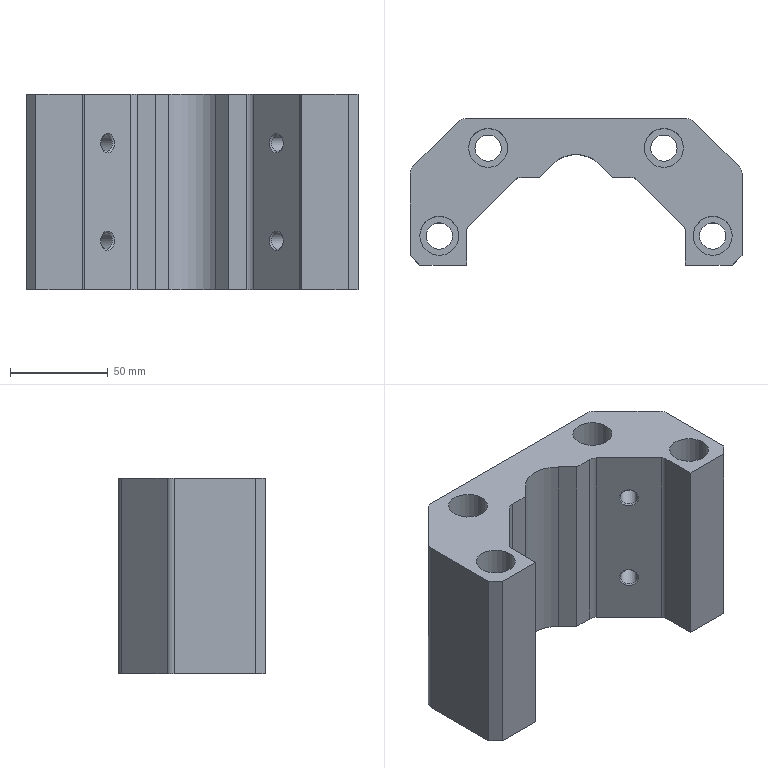Part | NX | features LB-9 2 | 1 solid | 52 faces | box 170 x 75 x 100 mm | volume 629709 mm3 | plane 23 | cylinder 21 | cone 8 | commonest cylinder face diameters 10 x6 8.506 x4 13.5 x4 20 x4 6 x2 34 x1
STEP:
#1=CARTESIAN_POINT('',(3387.594,-1089.122,888.716));
#2=VERTEX_POINT('',#1);
#3=CARTESIAN_POINT('',(3377.594,-1089.122,888.716));
#4=DIRECTION('',(0.,0.,1.));
#5=DIRECTION('',(1.,0.,0.));
#6=AXIS2_PLACEMENT_3D('',#3,#4,#5);
#7=CIRCLE('',#6,10.);
#8=EDGE_CURVE('',#2,#2,#7,.T.);
#9=ORIENTED_EDGE('',*,*,#8,.F.);
#10=EDGE_LOOP('',(#9));
#11=FACE_BOUND('',#10,.T.);
#12=CARTESIAN_POINT('',(3272.594,-1044.122,888.716));
#13=VERTEX_POINT('',#12);
#14=CARTESIAN_POINT('',(3262.594,-1044.122,888.716));
#15=DIRECTION('',(0.,0.,1.));
#16=DIRECTION('',(1.,0.,0.));
#17=AXIS2_PLACEMENT_3D('',#14,#15,#16);
#18=CIRCLE('',#17,10.);
#19=EDGE_CURVE('',#13,#13,#18,.T.);
#20=ORIENTED_EDGE('',*,*,#19,.F.);
#21=EDGE_LOOP('',(#20));
#22=FACE_BOUND('',#21,.T.);
#23=CARTESIAN_POINT('',(3362.594,-1044.122,888.716));
#24=VERTEX_POINT('',#23);
#25=CARTESIAN_POINT('',(3352.594,-1044.122,888.716));
#26=DIRECTION('',(0.,0.,1.));
#27=DIRECTION('',(1.,0.,0.));
#28=AXIS2_PLACEMENT_3D('',#25,#26,#27);
#29=CIRCLE('',#28,10.);
#30=EDGE_CURVE('',#24,#24,#29,.T.);
#31=ORIENTED_EDGE('',*,*,#30,.F.);
#32=EDGE_LOOP('',(#31));
#33=FACE_BOUND('',#32,.T.);
#34=CARTESIAN_POINT('',(3247.594,-1089.122,888.716));
#35=VERTEX_POINT('',#34);
#36=CARTESIAN_POINT('',(3237.594,-1089.122,888.716));
#37=DIRECTION('',(0.,0.,1.));
#38=DIRECTION('',(1.,0.,0.));
#39=AXIS2_PLACEMENT_3D('',#36,#37,#38);
#40=CIRCLE('',#39,10.);
#41=EDGE_CURVE('',#35,#35,#40,.T.);
#42=ORIENTED_EDGE('',*,*,#41,.F.);
#43=EDGE_LOOP('',(#42));
#44=FACE_BOUND('',#43,.T.);
#45=CARTESIAN_POINT('',(3392.594,-1099.122,888.716));
#46=VERTEX_POINT('',#45);
#47=CARTESIAN_POINT('',(3392.594,-1057.406,888.716));
#48=VERTEX_POINT('',#47);
#49=CARTESIAN_POINT('',(3392.594,-1019.122,888.716));
#50=DIRECTION('',(0.,1.,0.));
#51=VECTOR('',#50,1000.);
#52=LINE('',#49,#51);
#53=EDGE_CURVE('',#46,#48,#52,.T.);
#54=ORIENTED_EDGE('',*,*,#53,.T.);
#55=CARTESIAN_POINT('',(3391.129,-1053.871,888.716));
#56=VERTEX_POINT('',#55);
#57=CARTESIAN_POINT('',(3387.594,-1057.406,888.716));
#58=DIRECTION('',(0.,0.,1.));
#59=DIRECTION('',(1.,0.,0.));
#60=AXIS2_PLACEMENT_3D('',#57,#58,#59);
#61=CIRCLE('',#60,5.);
#62=EDGE_CURVE('',#48,#56,#61,.T.);
#63=ORIENTED_EDGE('',*,*,#62,.T.);
#64=CARTESIAN_POINT('',(3367.845,-1030.587,888.716));
#65=VERTEX_POINT('',#64);
#66=CARTESIAN_POINT('',(3138.314,-801.055,888.716));
#67=DIRECTION('',(-0.7071,0.7071,0.));
#68=VECTOR('',#67,1000.);
#69=LINE('',#66,#68);
#70=EDGE_CURVE('',#56,#65,#69,.T.);
#71=ORIENTED_EDGE('',*,*,#70,.T.);
#72=CARTESIAN_POINT('',(3364.31,-1029.122,888.716));
#73=VERTEX_POINT('',#72);
#74=CARTESIAN_POINT('',(3364.31,-1034.122,888.716));
#75=DIRECTION('',(0.,0.,1.));
#76=DIRECTION('',(1.,0.,0.));
#77=AXIS2_PLACEMENT_3D('',#74,#75,#76);
#78=CIRCLE('',#77,5.);
#79=EDGE_CURVE('',#65,#73,#78,.T.);
#80=ORIENTED_EDGE('',*,*,#79,.T.);
#81=CARTESIAN_POINT('',(3250.878,-1029.122,888.716));
#82=VERTEX_POINT('',#81);
#83=CARTESIAN_POINT('',(3237.747,-1029.122,888.716));
#84=DIRECTION('',(1.,0.,0.));
#85=VECTOR('',#84,1000.);
#86=LINE('',#83,#85);
#87=EDGE_CURVE('',#82,#73,#86,.T.);
#88=ORIENTED_EDGE('',*,*,#87,.F.);
#89=CARTESIAN_POINT('',(3247.343,-1030.587,888.716));
#90=VERTEX_POINT('',#89);
#91=CARTESIAN_POINT('',(3250.878,-1034.122,888.716));
#92=DIRECTION('',(0.,0.,1.));
#93=DIRECTION('',(1.,0.,0.));
#94=AXIS2_PLACEMENT_3D('',#91,#92,#93);
#95=CIRCLE('',#94,5.);
#96=EDGE_CURVE('',#82,#90,#95,.T.);
#97=ORIENTED_EDGE('',*,*,#96,.T.);
#98=CARTESIAN_POINT('',(3224.058,-1053.871,888.716));
#99=VERTEX_POINT('',#98);
#100=CARTESIAN_POINT('',(3407.027,-870.902,888.716));
#101=DIRECTION('',(-0.7071,-0.7071,0.));
#102=VECTOR('',#101,1000.);
#103=LINE('',#100,#102);
#104=EDGE_CURVE('',#90,#99,#103,.T.);
#105=ORIENTED_EDGE('',*,*,#104,.T.);
#106=CARTESIAN_POINT('',(3222.594,-1057.406,888.716));
#107=VERTEX_POINT('',#106);
#108=CARTESIAN_POINT('',(3227.594,-1057.406,888.716));
#109=DIRECTION('',(0.,0.,1.));
#110=DIRECTION('',(1.,0.,0.));
#111=AXIS2_PLACEMENT_3D('',#108,#109,#110);
#112=CIRCLE('',#111,5.);
#113=EDGE_CURVE('',#99,#107,#112,.T.);
#114=ORIENTED_EDGE('',*,*,#113,.T.);
#115=CARTESIAN_POINT('',(3222.594,-1099.122,888.716));
#116=VERTEX_POINT('',#115);
#117=CARTESIAN_POINT('',(3222.594,-701.622,888.716));
#118=DIRECTION('',(0.,-1.,0.));
#119=VECTOR('',#118,1000.);
#120=LINE('',#117,#119);
#121=EDGE_CURVE('',#107,#116,#120,.T.);
#122=ORIENTED_EDGE('',*,*,#121,.T.);
#123=CARTESIAN_POINT('',(3227.594,-1104.122,888.716));
#124=VERTEX_POINT('',#123);
#125=CARTESIAN_POINT('',(3023.92,-900.449,888.716));
#126=DIRECTION('',(0.7071,-0.7071,0.));
#127=VECTOR('',#126,1000.);
#128=LINE('',#125,#127);
#129=EDGE_CURVE('',#116,#124,#128,.T.);
#130=ORIENTED_EDGE('',*,*,#129,.T.);
#131=CARTESIAN_POINT('',(3251.594,-1104.122,888.716));
#132=VERTEX_POINT('',#131);
#133=CARTESIAN_POINT('',(4385.094,-1104.122,888.716));
#134=DIRECTION('',(-1.,0.,0.));
#135=VECTOR('',#134,1000.);
#136=LINE('',#133,#135);
#137=EDGE_CURVE('',#132,#124,#136,.T.);
#138=ORIENTED_EDGE('',*,*,#137,.F.);
#139=CARTESIAN_POINT('',(3251.594,-1086.365,888.716));
#140=VERTEX_POINT('',#139);
#141=CARTESIAN_POINT('',(3251.594,-701.622,888.716));
#142=DIRECTION('',(0.,-1.,0.));
#143=VECTOR('',#142,1000.);
#144=LINE('',#141,#143);
#145=EDGE_CURVE('',#140,#132,#144,.T.);
#146=ORIENTED_EDGE('',*,*,#145,.F.);
#147=CARTESIAN_POINT('',(3252.473,-1084.243,888.716));
#148=VERTEX_POINT('',#147);
#149=CARTESIAN_POINT('',(3254.594,-1086.365,888.716));
#150=DIRECTION('',(0.,0.,-1.));
#151=DIRECTION('',(1.,0.,0.));
#152=AXIS2_PLACEMENT_3D('',#149,#150,#151);
#153=CIRCLE('',#152,3.);
#154=EDGE_CURVE('',#140,#148,#153,.T.);
#155=ORIENTED_EDGE('',*,*,#154,.T.);
#156=CARTESIAN_POINT('',(3276.129,-1060.587,888.716));
#157=VERTEX_POINT('',#156);
#158=CARTESIAN_POINT('',(3428.92,-907.796,888.716));
#159=DIRECTION('',(-0.7071,-0.7071,0.));
#160=VECTOR('',#159,1000.);
#161=LINE('',#158,#160);
#162=EDGE_CURVE('',#157,#148,#161,.T.);
#163=ORIENTED_EDGE('',*,*,#162,.F.);
#164=CARTESIAN_POINT('',(3279.665,-1059.122,888.716));
#165=VERTEX_POINT('',#164);
#166=CARTESIAN_POINT('',(3279.665,-1064.122,888.716));
#167=DIRECTION('',(0.,0.,-1.));
#168=DIRECTION('',(1.,0.,0.));
#169=AXIS2_PLACEMENT_3D('',#166,#167,#168);
#170=CIRCLE('',#169,5.);
#171=EDGE_CURVE('',#157,#165,#170,.T.);
#172=ORIENTED_EDGE('',*,*,#171,.T.);
#173=CARTESIAN_POINT('',(3288.908,-1059.122,888.716));
#174=VERTEX_POINT('',#173);
#175=CARTESIAN_POINT('',(3237.747,-1059.122,888.716));
#176=DIRECTION('',(-1.,0.,0.));
#177=VECTOR('',#176,1000.);
#178=LINE('',#175,#177);
#179=EDGE_CURVE('',#174,#165,#178,.T.);
#180=ORIENTED_EDGE('',*,*,#179,.F.);
#181=CARTESIAN_POINT('',(3295.573,-1052.457,888.716));
#182=VERTEX_POINT('',#181);
#183=CARTESIAN_POINT('',(3442.077,-905.952,888.716));
#184=DIRECTION('',(0.7071,0.7071,0.));
#185=VECTOR('',#184,1000.);
#186=LINE('',#183,#185);
#187=EDGE_CURVE('',#174,#182,#186,.T.);
#188=ORIENTED_EDGE('',*,*,#187,.T.);
#189=CARTESIAN_POINT('',(3319.615,-1052.457,888.716));
#190=VERTEX_POINT('',#189);
#191=CARTESIAN_POINT('',(3307.594,-1064.477,888.716));
#192=DIRECTION('',(0.,0.,1.));
#193=DIRECTION('',(1.,0.,0.));
#194=AXIS2_PLACEMENT_3D('',#191,#192,#193);
#195=CIRCLE('',#194,17.);
#196=EDGE_CURVE('',#190,#182,#195,.T.);
#197=ORIENTED_EDGE('',*,*,#196,.F.);
#198=CARTESIAN_POINT('',(3326.28,-1059.122,888.716));
#199=VERTEX_POINT('',#198);
#200=CARTESIAN_POINT('',(3103.264,-836.105,888.716));
#201=DIRECTION('',(0.7071,-0.7071,0.));
#202=VECTOR('',#201,1000.);
#203=LINE('',#200,#202);
#204=EDGE_CURVE('',#190,#199,#203,.T.);
#205=ORIENTED_EDGE('',*,*,#204,.T.);
#206=CARTESIAN_POINT('',(3335.523,-1059.122,888.716));
#207=VERTEX_POINT('',#206);
#208=CARTESIAN_POINT('',(3237.747,-1059.122,888.716));
#209=DIRECTION('',(-1.,0.,0.));
#210=VECTOR('',#209,1000.);
#211=LINE('',#208,#210);
#212=EDGE_CURVE('',#207,#199,#211,.T.);
#213=ORIENTED_EDGE('',*,*,#212,.F.);
#214=CARTESIAN_POINT('',(3339.058,-1060.587,888.716));
#215=VERTEX_POINT('',#214);
#216=CARTESIAN_POINT('',(3335.523,-1064.122,888.716));
#217=DIRECTION('',(0.,0.,-1.));
#218=DIRECTION('',(1.,0.,0.));
#219=AXIS2_PLACEMENT_3D('',#216,#217,#218);
#220=CIRCLE('',#219,5.);
#221=EDGE_CURVE('',#207,#215,#220,.T.);
#222=ORIENTED_EDGE('',*,*,#221,.T.);
#223=CARTESIAN_POINT('',(3362.715,-1084.243,888.716));
#224=VERTEX_POINT('',#223);
#225=CARTESIAN_POINT('',(3347.594,-1069.122,888.716));
#226=DIRECTION('',(-0.7071,0.7071,0.));
#227=VECTOR('',#226,1000.);
#228=LINE('',#225,#227);
#229=EDGE_CURVE('',#224,#215,#228,.T.);
#230=ORIENTED_EDGE('',*,*,#229,.F.);
#231=CARTESIAN_POINT('',(3363.594,-1086.365,888.716));
#232=VERTEX_POINT('',#231);
#233=CARTESIAN_POINT('',(3360.594,-1086.365,888.716));
#234=DIRECTION('',(0.,0.,-1.));
#235=DIRECTION('',(1.,0.,0.));
#236=AXIS2_PLACEMENT_3D('',#233,#234,#235);
#237=CIRCLE('',#236,3.);
#238=EDGE_CURVE('',#224,#232,#237,.T.);
#239=ORIENTED_EDGE('',*,*,#238,.T.);
#240=CARTESIAN_POINT('',(3363.594,-1104.122,888.716));
#241=VERTEX_POINT('',#240);
#242=CARTESIAN_POINT('',(3363.594,-1061.622,888.716));
#243=DIRECTION('',(0.,-1.,0.));
#244=VECTOR('',#243,1000.);
#245=LINE('',#242,#244);
#246=EDGE_CURVE('',#232,#241,#245,.T.);
#247=ORIENTED_EDGE('',*,*,#246,.T.);
#248=CARTESIAN_POINT('',(3387.594,-1104.122,888.716));
#249=VERTEX_POINT('',#248);
#250=CARTESIAN_POINT('',(4387.594,-1104.122,888.716));
#251=DIRECTION('',(-1.,0.,0.));
#252=VECTOR('',#251,1000.);
#253=LINE('',#250,#252);
#254=EDGE_CURVE('',#249,#241,#253,.T.);
#255=ORIENTED_EDGE('',*,*,#254,.F.);
#256=CARTESIAN_POINT('',(3521.42,-970.296,888.716));
#257=DIRECTION('',(0.7071,0.7071,0.));
#258=VECTOR('',#257,1000.);
#259=LINE('',#256,#258);
#260=EDGE_CURVE('',#249,#46,#259,.T.);
#261=ORIENTED_EDGE('',*,*,#260,.T.);
#262=EDGE_LOOP('',(#54,#63,#71,#80,#88,#97,#105,#114,#122,#130,#138,#146,#155,#163,#172,#180,#188,#197,#205,#213,#222,#230,#239,#247,#255,#261));
#263=FACE_BOUND('',#262,.T.);
#264=CARTESIAN_POINT('',(3237.747,-701.622,888.716));
#265=DIRECTION('',(0.,0.,1.));
#266=DIRECTION('',(-1.,0.,0.));
#267=AXIS2_PLACEMENT_3D('',#264,#265,#266);
#268=PLANE('',#267);
#269=ADVANCED_FACE('',(#11,#22,#33,#44,#263),#268,.T.);
#270=CARTESIAN_POINT('',(3384.344,-1089.122,788.716));
#271=VERTEX_POINT('',#270);
#272=CARTESIAN_POINT('',(3377.594,-1089.122,788.716));
#273=DIRECTION('',(0.,0.,1.));
#274=DIRECTION('',(1.,0.,0.));
#275=AXIS2_PLACEMENT_3D('',#272,#273,#274);
#276=CIRCLE('',#275,6.75);
#277=EDGE_CURVE('',#271,#271,#276,.T.);
#278=ORIENTED_EDGE('',*,*,#277,.T.);
#279=EDGE_LOOP('',(#278));
#280=FACE_BOUND('',#279,.T.);
#281=CARTESIAN_POINT('',(3269.344,-1044.122,788.716));
#282=VERTEX_POINT('',#281);
#283=CARTESIAN_POINT('',(3262.594,-1044.122,788.716));
#284=DIRECTION('',(0.,0.,1.));
#285=DIRECTION('',(1.,0.,0.));
#286=AXIS2_PLACEMENT_3D('',#283,#284,#285);
#287=CIRCLE('',#286,6.75);
#288=EDGE_CURVE('',#282,#282,#287,.T.);
#289=ORIENTED_EDGE('',*,*,#288,.T.);
#290=EDGE_LOOP('',(#289));
#291=FACE_BOUND('',#290,.T.);
#292=CARTESIAN_POINT('',(3359.344,-1044.122,788.716));
#293=VERTEX_POINT('',#292);
#294=CARTESIAN_POINT('',(3352.594,-1044.122,788.716));
#295=DIRECTION('',(0.,0.,1.));
#296=DIRECTION('',(1.,0.,0.));
#297=AXIS2_PLACEMENT_3D('',#294,#295,#296);
#298=CIRCLE('',#297,6.75);
#299=EDGE_CURVE('',#293,#293,#298,.T.);
#300=ORIENTED_EDGE('',*,*,#299,.T.);
#301=EDGE_LOOP('',(#300));
#302=FACE_BOUND('',#301,.T.);
#303=CARTESIAN_POINT('',(3244.344,-1089.122,788.716));
#304=VERTEX_POINT('',#303);
#305=CARTESIAN_POINT('',(3237.594,-1089.122,788.716));
#306=DIRECTION('',(0.,0.,1.));
#307=DIRECTION('',(1.,0.,0.));
#308=AXIS2_PLACEMENT_3D('',#305,#306,#307);
#309=CIRCLE('',#308,6.75);
#310=EDGE_CURVE('',#304,#304,#309,.T.);
#311=ORIENTED_EDGE('',*,*,#310,.T.);
#312=EDGE_LOOP('',(#311));
#313=FACE_BOUND('',#312,.T.);
#314=CARTESIAN_POINT('',(3367.845,-1030.587,788.716));
#315=VERTEX_POINT('',#314);
#316=CARTESIAN_POINT('',(3391.129,-1053.871,788.716));
#317=VERTEX_POINT('',#316);
#318=CARTESIAN_POINT('',(3376.987,-1039.729,788.716));
#319=DIRECTION('',(0.7071,-0.7071,0.));
#320=VECTOR('',#319,1000.);
#321=LINE('',#318,#320);
#322=EDGE_CURVE('',#315,#317,#321,.T.);
#323=ORIENTED_EDGE('',*,*,#322,.T.);
#324=CARTESIAN_POINT('',(3392.594,-1057.406,788.716));
#325=VERTEX_POINT('',#324);
#326=CARTESIAN_POINT('',(3387.594,-1057.406,788.716));
#327=DIRECTION('',(0.,0.,-1.));
#328=DIRECTION('',(1.,0.,0.));
#329=AXIS2_PLACEMENT_3D('',#326,#327,#328);
#330=CIRCLE('',#329,5.);
#331=EDGE_CURVE('',#317,#325,#330,.T.);
#332=ORIENTED_EDGE('',*,*,#331,.T.);
#333=CARTESIAN_POINT('',(3392.594,-1099.122,788.716));
#334=VERTEX_POINT('',#333);
#335=CARTESIAN_POINT('',(3392.594,-299.122,788.716));
#336=DIRECTION('',(0.,-1.,0.));
#337=VECTOR('',#336,1000.);
#338=LINE('',#335,#337);
#339=EDGE_CURVE('',#325,#334,#338,.T.);
#340=ORIENTED_EDGE('',*,*,#339,.T.);
#341=CARTESIAN_POINT('',(3387.594,-1104.122,788.716));
#342=VERTEX_POINT('',#341);
#343=CARTESIAN_POINT('',(3392.594,-1099.122,788.716));
#344=DIRECTION('',(-0.7071,-0.7071,0.));
#345=VECTOR('',#344,1000.);
#346=LINE('',#343,#345);
#347=EDGE_CURVE('',#334,#342,#346,.T.);
#348=ORIENTED_EDGE('',*,*,#347,.T.);
#349=CARTESIAN_POINT('',(3363.594,-1104.122,788.716));
#350=VERTEX_POINT('',#349);
#351=CARTESIAN_POINT('',(3660.094,-1104.122,788.716));
#352=DIRECTION('',(1.,0.,0.));
#353=VECTOR('',#352,1000.);
#354=LINE('',#351,#353);
#355=EDGE_CURVE('',#350,#342,#354,.T.);
#356=ORIENTED_EDGE('',*,*,#355,.F.);
#357=CARTESIAN_POINT('',(3363.594,-1086.365,788.716));
#358=VERTEX_POINT('',#357);
#359=CARTESIAN_POINT('',(3363.594,-299.122,788.716));
#360=DIRECTION('',(0.,1.,0.));
#361=VECTOR('',#360,1000.);
#362=LINE('',#359,#361);
#363=EDGE_CURVE('',#350,#358,#362,.T.);
#364=ORIENTED_EDGE('',*,*,#363,.T.);
#365=CARTESIAN_POINT('',(3362.715,-1084.243,788.716));
#366=VERTEX_POINT('',#365);
#367=CARTESIAN_POINT('',(3360.594,-1086.365,788.716));
#368=DIRECTION('',(0.,0.,1.));
#369=DIRECTION('',(1.,0.,0.));
#370=AXIS2_PLACEMENT_3D('',#367,#368,#369);
#371=CIRCLE('',#370,3.);
#372=EDGE_CURVE('',#358,#366,#371,.T.);
#373=ORIENTED_EDGE('',*,*,#372,.T.);
#374=CARTESIAN_POINT('',(3339.058,-1060.587,788.716));
#375=VERTEX_POINT('',#374);
#376=CARTESIAN_POINT('',(3347.594,-1069.122,788.716));
#377=DIRECTION('',(-0.7071,0.7071,0.));
#378=VECTOR('',#377,1000.);
#379=LINE('',#376,#378);
#380=EDGE_CURVE('',#366,#375,#379,.T.);
#381=ORIENTED_EDGE('',*,*,#380,.T.);
#382=CARTESIAN_POINT('',(3335.523,-1059.122,788.716));
#383=VERTEX_POINT('',#382);
#384=CARTESIAN_POINT('',(3335.523,-1064.122,788.716));
#385=DIRECTION('',(0.,0.,1.));
#386=DIRECTION('',(1.,0.,0.));
#387=AXIS2_PLACEMENT_3D('',#384,#385,#386);
#388=CIRCLE('',#387,5.);
#389=EDGE_CURVE('',#375,#383,#388,.T.);
#390=ORIENTED_EDGE('',*,*,#389,.T.);
#391=CARTESIAN_POINT('',(3326.28,-1059.122,788.716));
#392=VERTEX_POINT('',#391);
#393=CARTESIAN_POINT('',(4922.709,-1059.122,788.716));
#394=DIRECTION('',(1.,0.,0.));
#395=VECTOR('',#394,1000.);
#396=LINE('',#393,#395);
#397=EDGE_CURVE('',#392,#383,#396,.T.);
#398=ORIENTED_EDGE('',*,*,#397,.F.);
#399=CARTESIAN_POINT('',(3319.615,-1052.457,788.716));
#400=VERTEX_POINT('',#399);
#401=CARTESIAN_POINT('',(3105.687,-838.529,788.716));
#402=DIRECTION('',(0.7071,-0.7071,0.));
#403=VECTOR('',#402,1000.);
#404=LINE('',#401,#403);
#405=EDGE_CURVE('',#400,#392,#404,.T.);
#406=ORIENTED_EDGE('',*,*,#405,.F.);
#407=CARTESIAN_POINT('',(3295.573,-1052.457,788.716));
#408=VERTEX_POINT('',#407);
#409=CARTESIAN_POINT('',(3307.594,-1064.477,788.716));
#410=DIRECTION('',(0.,0.,1.));
#411=DIRECTION('',(1.,0.,0.));
#412=AXIS2_PLACEMENT_3D('',#409,#410,#411);
#413=CIRCLE('',#412,17.);
#414=EDGE_CURVE('',#400,#408,#413,.T.);
#415=ORIENTED_EDGE('',*,*,#414,.T.);
#416=CARTESIAN_POINT('',(3288.908,-1059.122,788.716));
#417=VERTEX_POINT('',#416);
#418=CARTESIAN_POINT('',(3847.001,-501.029,788.716));
#419=DIRECTION('',(0.7071,0.7071,0.));
#420=VECTOR('',#419,1000.);
#421=LINE('',#418,#420);
#422=EDGE_CURVE('',#417,#408,#421,.T.);
#423=ORIENTED_EDGE('',*,*,#422,.F.);
#424=CARTESIAN_POINT('',(3279.665,-1059.122,788.716));
#425=VERTEX_POINT('',#424);
#426=CARTESIAN_POINT('',(4922.709,-1059.122,788.716));
#427=DIRECTION('',(1.,0.,0.));
#428=VECTOR('',#427,1000.);
#429=LINE('',#426,#428);
#430=EDGE_CURVE('',#425,#417,#429,.T.);
#431=ORIENTED_EDGE('',*,*,#430,.F.);
#432=CARTESIAN_POINT('',(3276.129,-1060.587,788.716));
#433=VERTEX_POINT('',#432);
#434=CARTESIAN_POINT('',(3279.665,-1064.122,788.716));
#435=DIRECTION('',(0.,0.,1.));
#436=DIRECTION('',(1.,0.,0.));
#437=AXIS2_PLACEMENT_3D('',#434,#435,#436);
#438=CIRCLE('',#437,5.);
#439=EDGE_CURVE('',#425,#433,#438,.T.);
#440=ORIENTED_EDGE('',*,*,#439,.T.);
#441=CARTESIAN_POINT('',(3252.473,-1084.243,788.716));
#442=VERTEX_POINT('',#441);
#443=CARTESIAN_POINT('',(3833.844,-502.872,788.716));
#444=DIRECTION('',(-0.7071,-0.7071,0.));
#445=VECTOR('',#444,1000.);
#446=LINE('',#443,#445);
#447=EDGE_CURVE('',#433,#442,#446,.T.);
#448=ORIENTED_EDGE('',*,*,#447,.T.);
#449=CARTESIAN_POINT('',(3251.594,-1086.365,788.716));
#450=VERTEX_POINT('',#449);
#451=CARTESIAN_POINT('',(3254.594,-1086.365,788.716));
#452=DIRECTION('',(0.,0.,1.));
#453=DIRECTION('',(1.,0.,0.));
#454=AXIS2_PLACEMENT_3D('',#451,#452,#453);
#455=CIRCLE('',#454,3.);
#456=EDGE_CURVE('',#442,#450,#455,.T.);
#457=ORIENTED_EDGE('',*,*,#456,.T.);
#458=CARTESIAN_POINT('',(3251.594,-1104.122,788.716));
#459=VERTEX_POINT('',#458);
#460=CARTESIAN_POINT('',(3251.594,-1061.622,788.716));
#461=DIRECTION('',(0.,1.,0.));
#462=VECTOR('',#461,1000.);
#463=LINE('',#460,#462);
#464=EDGE_CURVE('',#459,#450,#463,.T.);
#465=ORIENTED_EDGE('',*,*,#464,.F.);
#466=CARTESIAN_POINT('',(3227.594,-1104.122,788.716));
#467=VERTEX_POINT('',#466);
#468=CARTESIAN_POINT('',(4385.094,-1104.122,788.716));
#469=DIRECTION('',(-1.,0.,0.));
#470=VECTOR('',#469,1000.);
#471=LINE('',#468,#470);
#472=EDGE_CURVE('',#459,#467,#471,.T.);
#473=ORIENTED_EDGE('',*,*,#472,.T.);
#474=CARTESIAN_POINT('',(3222.594,-1099.122,788.716));
#475=VERTEX_POINT('',#474);
#476=CARTESIAN_POINT('',(3227.594,-1104.122,788.716));
#477=DIRECTION('',(-0.7071,0.7071,0.));
#478=VECTOR('',#477,1000.);
#479=LINE('',#476,#478);
#480=EDGE_CURVE('',#467,#475,#479,.T.);
#481=ORIENTED_EDGE('',*,*,#480,.T.);
#482=CARTESIAN_POINT('',(3222.594,-1057.406,788.716));
#483=VERTEX_POINT('',#482);
#484=CARTESIAN_POINT('',(3222.594,-299.122,788.716));
#485=DIRECTION('',(0.,-1.,0.));
#486=VECTOR('',#485,1000.);
#487=LINE('',#484,#486);
#488=EDGE_CURVE('',#483,#475,#487,.T.);
#489=ORIENTED_EDGE('',*,*,#488,.F.);
#490=CARTESIAN_POINT('',(3224.058,-1053.871,788.716));
#491=VERTEX_POINT('',#490);
#492=CARTESIAN_POINT('',(3227.594,-1057.406,788.716));
#493=DIRECTION('',(0.,0.,-1.));
#494=DIRECTION('',(1.,0.,0.));
#495=AXIS2_PLACEMENT_3D('',#492,#493,#494);
#496=CIRCLE('',#495,5.);
#497=EDGE_CURVE('',#483,#491,#496,.T.);
#498=ORIENTED_EDGE('',*,*,#497,.T.);
#499=CARTESIAN_POINT('',(3247.343,-1030.587,788.716));
#500=VERTEX_POINT('',#499);
#501=CARTESIAN_POINT('',(3233.201,-1044.729,788.716));
#502=DIRECTION('',(0.7071,0.7071,0.));
#503=VECTOR('',#502,1000.);
#504=LINE('',#501,#503);
#505=EDGE_CURVE('',#491,#500,#504,.T.);
#506=ORIENTED_EDGE('',*,*,#505,.T.);
#507=CARTESIAN_POINT('',(3250.878,-1029.122,788.716));
#508=VERTEX_POINT('',#507);
#509=CARTESIAN_POINT('',(3250.878,-1034.122,788.716));
#510=DIRECTION('',(0.,0.,-1.));
#511=DIRECTION('',(1.,0.,0.));
#512=AXIS2_PLACEMENT_3D('',#509,#510,#511);
#513=CIRCLE('',#512,5.);
#514=EDGE_CURVE('',#500,#508,#513,.T.);
#515=ORIENTED_EDGE('',*,*,#514,.T.);
#516=CARTESIAN_POINT('',(3364.31,-1029.122,788.716));
#517=VERTEX_POINT('',#516);
#518=CARTESIAN_POINT('',(3645.094,-1029.122,788.716));
#519=DIRECTION('',(1.,0.,0.));
#520=VECTOR('',#519,1000.);
#521=LINE('',#518,#520);
#522=EDGE_CURVE('',#508,#517,#521,.T.);
#523=ORIENTED_EDGE('',*,*,#522,.T.);
#524=CARTESIAN_POINT('',(3364.31,-1034.122,788.716));
#525=DIRECTION('',(0.,0.,-1.));
#526=DIRECTION('',(1.,0.,0.));
#527=AXIS2_PLACEMENT_3D('',#524,#525,#526);
#528=CIRCLE('',#527,5.);
#529=EDGE_CURVE('',#517,#315,#528,.T.);
#530=ORIENTED_EDGE('',*,*,#529,.T.);
#531=EDGE_LOOP('',(#323,#332,#340,#348,#356,#364,#373,#381,#390,#398,#406,#415,#423,#431,#440,#448,#457,#465,#473,#481,#489,#498,#506,#515,#523,#530));
#532=FACE_BOUND('',#531,.T.);
#533=CARTESIAN_POINT('',(3645.094,-299.122,788.716));
#534=DIRECTION('',(0.,0.,1.));
#535=DIRECTION('',(-1.,0.,0.));
#536=AXIS2_PLACEMENT_3D('',#533,#534,#535);
#537=PLANE('',#536);
#538=ADVANCED_FACE('',(#280,#291,#302,#313,#532),#537,.F.);
#539=CARTESIAN_POINT('',(3326.28,-1059.122,473.116));
#540=DIRECTION('',(0.,0.,1.));
#541=VECTOR('',#540,1000.);
#542=LINE('',#539,#541);
#543=EDGE_CURVE('',#392,#199,#542,.T.);
#544=ORIENTED_EDGE('',*,*,#543,.F.);
#545=ORIENTED_EDGE('',*,*,#397,.T.);
#546=CARTESIAN_POINT('',(3335.523,-1059.122,473.116));
#547=DIRECTION('',(0.,0.,1.));
#548=VECTOR('',#547,1000.);
#549=LINE('',#546,#548);
#550=EDGE_CURVE('',#383,#207,#549,.T.);
#551=ORIENTED_EDGE('',*,*,#550,.T.);
#552=ORIENTED_EDGE('',*,*,#212,.T.);
#553=EDGE_LOOP('',(#544,#545,#551,#552));
#554=FACE_BOUND('',#553,.T.);
#555=CARTESIAN_POINT('',(4922.709,-1059.122,473.116));
#556=DIRECTION('',(0.,1.,0.));
#557=DIRECTION('',(0.,0.,1.));
#558=AXIS2_PLACEMENT_3D('',#555,#556,#557);
#559=PLANE('',#558);
#560=ADVANCED_FACE('',(#554),#559,.F.);
#561=CARTESIAN_POINT('',(3288.908,-1059.122,473.116));
#562=DIRECTION('',(0.,0.,-1.));
#563=VECTOR('',#562,1000.);
#564=LINE('',#561,#563);
#565=EDGE_CURVE('',#174,#417,#564,.T.);
#566=ORIENTED_EDGE('',*,*,#565,.F.);
#567=ORIENTED_EDGE('',*,*,#179,.T.);
#568=CARTESIAN_POINT('',(3279.665,-1059.122,768.716));
#569=DIRECTION('',(0.,0.,-1.));
#570=VECTOR('',#569,1000.);
#571=LINE('',#568,#570);
#572=EDGE_CURVE('',#165,#425,#571,.T.);
#573=ORIENTED_EDGE('',*,*,#572,.T.);
#574=ORIENTED_EDGE('',*,*,#430,.T.);
#575=EDGE_LOOP('',(#566,#567,#573,#574));
#576=FACE_BOUND('',#575,.T.);
#577=CARTESIAN_POINT('',(4922.709,-1059.122,473.116));
#578=DIRECTION('',(0.,1.,0.));
#579=DIRECTION('',(0.,0.,1.));
#580=AXIS2_PLACEMENT_3D('',#577,#578,#579);
#581=PLANE('',#580);
#582=ADVANCED_FACE('',(#576),#581,.F.);
#583=ORIENTED_EDGE('',*,*,#87,.T.);
#584=CARTESIAN_POINT('',(3364.31,-1029.122,788.716));
#585=DIRECTION('',(0.,0.,-1.));
#586=VECTOR('',#585,1000.);
#587=LINE('',#584,#586);
#588=EDGE_CURVE('',#73,#517,#587,.T.);
#589=ORIENTED_EDGE('',*,*,#588,.T.);
#590=ORIENTED_EDGE('',*,*,#522,.F.);
#591=CARTESIAN_POINT('',(3250.878,-1029.122,888.716));
#592=DIRECTION('',(0.,0.,1.));
#593=VECTOR('',#592,1000.);
#594=LINE('',#591,#593);
#595=EDGE_CURVE('',#508,#82,#594,.T.);
#596=ORIENTED_EDGE('',*,*,#595,.T.);
#597=EDGE_LOOP('',(#583,#589,#590,#596));
#598=FACE_BOUND('',#597,.T.);
#599=CARTESIAN_POINT('',(4847.709,-1029.122,913.116));
#600=DIRECTION('',(0.,-1.,0.));
#601=DIRECTION('',(0.,0.,-1.));
#602=AXIS2_PLACEMENT_3D('',#599,#600,#601);
#603=PLANE('',#602);
#604=ADVANCED_FACE('',(#598),#603,.F.);
#605=CARTESIAN_POINT('',(3266.887,-1069.829,817.252));
#606=VERTEX_POINT('',#605);
#607=CARTESIAN_POINT('',(3264.387,-1072.329,813.716));
#608=DIRECTION('',(0.7071,-0.7071,0.));
#609=DIRECTION('',(0.5,0.5,0.7071));
#610=AXIS2_PLACEMENT_3D('',#607,#608,#609);
#611=CIRCLE('',#610,5.);
#612=EDGE_CURVE('',#606,#606,#611,.T.);
#613=ORIENTED_EDGE('',*,*,#612,.F.);
#614=EDGE_LOOP('',(#613));
#615=FACE_BOUND('',#614,.T.);
#616=CARTESIAN_POINT('',(3266.887,-1069.829,867.252));
#617=VERTEX_POINT('',#616);
#618=CARTESIAN_POINT('',(3264.387,-1072.329,863.716));
#619=DIRECTION('',(0.7071,-0.7071,0.));
#620=DIRECTION('',(0.5,0.5,0.7071));
#621=AXIS2_PLACEMENT_3D('',#618,#619,#620);
#622=CIRCLE('',#621,5.);
#623=EDGE_CURVE('',#617,#617,#622,.T.);
#624=ORIENTED_EDGE('',*,*,#623,.F.);
#625=EDGE_LOOP('',(#624));
#626=FACE_BOUND('',#625,.T.);
#627=ORIENTED_EDGE('',*,*,#162,.T.);
#628=CARTESIAN_POINT('',(3252.473,-1084.243,788.716));
#629=DIRECTION('',(0.,0.,-1.));
#630=VECTOR('',#629,1000.);
#631=LINE('',#628,#630);
#632=EDGE_CURVE('',#148,#442,#631,.T.);
#633=ORIENTED_EDGE('',*,*,#632,.T.);
#634=ORIENTED_EDGE('',*,*,#447,.F.);
#635=CARTESIAN_POINT('',(3276.129,-1060.587,888.716));
#636=DIRECTION('',(0.,0.,1.));
#637=VECTOR('',#636,1000.);
#638=LINE('',#635,#637);
#639=EDGE_CURVE('',#433,#157,#638,.T.);
#640=ORIENTED_EDGE('',*,*,#639,.T.);
#641=EDGE_LOOP('',(#627,#633,#634,#640));
#642=FACE_BOUND('',#641,.T.);
#643=CARTESIAN_POINT('',(3282.594,-1054.122,473.116));
#644=DIRECTION('',(-0.7071,0.7071,0.));
#645=DIRECTION('',(0.,0.,1.));
#646=AXIS2_PLACEMENT_3D('',#643,#644,#645);
#647=PLANE('',#646);
#648=ADVANCED_FACE('',(#615,#626,#642),#647,.F.);
#649=CARTESIAN_POINT('',(3353.301,-1074.829,810.181));
#650=VERTEX_POINT('',#649);
#651=CARTESIAN_POINT('',(3350.801,-1072.329,813.716));
#652=DIRECTION('',(-0.7071,-0.7071,0.));
#653=DIRECTION('',(0.5,-0.5,-0.7071));
#654=AXIS2_PLACEMENT_3D('',#651,#652,#653);
#655=CIRCLE('',#654,5.);
#656=EDGE_CURVE('',#650,#650,#655,.T.);
#657=ORIENTED_EDGE('',*,*,#656,.F.);
#658=EDGE_LOOP('',(#657));
#659=FACE_BOUND('',#658,.T.);
#660=CARTESIAN_POINT('',(3353.301,-1074.829,860.181));
#661=VERTEX_POINT('',#660);
#662=CARTESIAN_POINT('',(3350.801,-1072.329,863.716));
#663=DIRECTION('',(-0.7071,-0.7071,0.));
#664=DIRECTION('',(0.5,-0.5,-0.7071));
#665=AXIS2_PLACEMENT_3D('',#662,#663,#664);
#666=CIRCLE('',#665,5.);
#667=EDGE_CURVE('',#661,#661,#666,.T.);
#668=ORIENTED_EDGE('',*,*,#667,.F.);
#669=EDGE_LOOP('',(#668));
#670=FACE_BOUND('',#669,.T.);
#671=ORIENTED_EDGE('',*,*,#380,.F.);
#672=CARTESIAN_POINT('',(3362.715,-1084.243,833.716));
#673=DIRECTION('',(0.,0.,1.));
#674=VECTOR('',#673,1000.);
#675=LINE('',#672,#674);
#676=EDGE_CURVE('',#366,#224,#675,.T.);
#677=ORIENTED_EDGE('',*,*,#676,.T.);
#678=ORIENTED_EDGE('',*,*,#229,.T.);
#679=CARTESIAN_POINT('',(3339.058,-1060.587,833.716));
#680=DIRECTION('',(0.,0.,-1.));
#681=VECTOR('',#680,1000.);
#682=LINE('',#679,#681);
#683=EDGE_CURVE('',#215,#375,#682,.T.);
#684=ORIENTED_EDGE('',*,*,#683,.T.);
#685=EDGE_LOOP('',(#671,#677,#678,#684));
#686=FACE_BOUND('',#685,.T.);
#687=CARTESIAN_POINT('',(3347.594,-1069.122,833.716));
#688=DIRECTION('',(-0.7071,-0.7071,0.));
#689=DIRECTION('',(-0.7071,0.7071,0.));
#690=AXIS2_PLACEMENT_3D('',#687,#688,#689);
#691=PLANE('',#690);
#692=ADVANCED_FACE('',(#659,#670,#686),#691,.T.);
#693=ORIENTED_EDGE('',*,*,#355,.T.);
#694=CARTESIAN_POINT('',(3387.594,-1104.122,888.716));
#695=DIRECTION('',(0.,0.,1.));
#696=VECTOR('',#695,1000.);
#697=LINE('',#694,#696);
#698=EDGE_CURVE('',#342,#249,#697,.T.);
#699=ORIENTED_EDGE('',*,*,#698,.T.);
#700=ORIENTED_EDGE('',*,*,#254,.T.);
#701=CARTESIAN_POINT('',(3363.594,-1104.122,828.716));
#702=DIRECTION('',(0.,0.,-1.));
#703=VECTOR('',#702,1000.);
#704=LINE('',#701,#703);
#705=EDGE_CURVE('',#241,#350,#704,.T.);
#706=ORIENTED_EDGE('',*,*,#705,.T.);
#707=EDGE_LOOP('',(#693,#699,#700,#706));
#708=FACE_BOUND('',#707,.T.);
#709=CARTESIAN_POINT('',(4387.594,-1104.122,748.716));
#710=DIRECTION('',(0.,-1.,0.));
#711=DIRECTION('',(-1.,0.,0.));
#712=AXIS2_PLACEMENT_3D('',#709,#710,#711);
#713=PLANE('',#712);
#714=ADVANCED_FACE('',(#708),#713,.T.);
#715=ORIENTED_EDGE('',*,*,#339,.F.);
#716=CARTESIAN_POINT('',(3392.594,-1057.406,888.716));
#717=DIRECTION('',(0.,0.,1.));
#718=VECTOR('',#717,1000.);
#719=LINE('',#716,#718);
#720=EDGE_CURVE('',#325,#48,#719,.T.);
#721=ORIENTED_EDGE('',*,*,#720,.T.);
#722=ORIENTED_EDGE('',*,*,#53,.F.);
#723=CARTESIAN_POINT('',(3392.594,-1099.122,788.716));
#724=DIRECTION('',(0.,0.,-1.));
#725=VECTOR('',#724,1000.);
#726=LINE('',#723,#725);
#727=EDGE_CURVE('',#46,#334,#726,.T.);
#728=ORIENTED_EDGE('',*,*,#727,.T.);
#729=EDGE_LOOP('',(#715,#721,#722,#728));
#730=FACE_BOUND('',#729,.T.);
#731=CARTESIAN_POINT('',(3392.594,-1019.122,958.116));
#732=DIRECTION('',(-1.,0.,0.));
#733=DIRECTION('',(0.,0.,-1.));
#734=AXIS2_PLACEMENT_3D('',#731,#732,#733);
#735=PLANE('',#734);
#736=ADVANCED_FACE('',(#730),#735,.F.);
#737=ORIENTED_EDGE('',*,*,#246,.F.);
#738=CARTESIAN_POINT('',(3363.594,-1086.365,828.716));
#739=DIRECTION('',(0.,0.,-1.));
#740=VECTOR('',#739,1000.);
#741=LINE('',#738,#740);
#742=EDGE_CURVE('',#232,#358,#741,.T.);
#743=ORIENTED_EDGE('',*,*,#742,.T.);
#744=ORIENTED_EDGE('',*,*,#363,.F.);
#745=ORIENTED_EDGE('',*,*,#705,.F.);
#746=EDGE_LOOP('',(#737,#743,#744,#745));
#747=FACE_BOUND('',#746,.T.);
#748=CARTESIAN_POINT('',(3363.594,-1061.622,828.716));
#749=DIRECTION('',(1.,0.,0.));
#750=DIRECTION('',(0.,0.,1.));
#751=AXIS2_PLACEMENT_3D('',#748,#749,#750);
#752=PLANE('',#751);
#753=ADVANCED_FACE('',(#747),#752,.F.);
#754=ORIENTED_EDGE('',*,*,#121,.F.);
#755=CARTESIAN_POINT('',(3222.594,-1057.406,958.116));
#756=DIRECTION('',(0.,0.,-1.));
#757=VECTOR('',#756,1000.);
#758=LINE('',#755,#757);
#759=EDGE_CURVE('',#107,#483,#758,.T.);
#760=ORIENTED_EDGE('',*,*,#759,.T.);
#761=ORIENTED_EDGE('',*,*,#488,.T.);
#762=CARTESIAN_POINT('',(3222.594,-1099.122,958.116));
#763=DIRECTION('',(0.,0.,1.));
#764=VECTOR('',#763,1000.);
#765=LINE('',#762,#764);
#766=EDGE_CURVE('',#475,#116,#765,.T.);
#767=ORIENTED_EDGE('',*,*,#766,.T.);
#768=EDGE_LOOP('',(#754,#760,#761,#767));
#769=FACE_BOUND('',#768,.T.);
#770=CARTESIAN_POINT('',(3222.594,-1019.122,958.116));
#771=DIRECTION('',(-1.,0.,0.));
#772=DIRECTION('',(0.,0.,-1.));
#773=AXIS2_PLACEMENT_3D('',#770,#771,#772);
#774=PLANE('',#773);
#775=ADVANCED_FACE('',(#769),#774,.T.);
#776=ORIENTED_EDGE('',*,*,#137,.T.);
#777=CARTESIAN_POINT('',(3227.594,-1104.122,748.716));
#778=DIRECTION('',(0.,0.,-1.));
#779=VECTOR('',#778,1000.);
#780=LINE('',#777,#779);
#781=EDGE_CURVE('',#124,#467,#780,.T.);
#782=ORIENTED_EDGE('',*,*,#781,.T.);
#783=ORIENTED_EDGE('',*,*,#472,.F.);
#784=CARTESIAN_POINT('',(3251.594,-1104.122,748.716));
#785=DIRECTION('',(0.,0.,-1.));
#786=VECTOR('',#785,1000.);
#787=LINE('',#784,#786);
#788=EDGE_CURVE('',#132,#459,#787,.T.);
#789=ORIENTED_EDGE('',*,*,#788,.F.);
#790=EDGE_LOOP('',(#776,#782,#783,#789));
#791=FACE_BOUND('',#790,.T.);
#792=CARTESIAN_POINT('',(4385.094,-1104.122,748.716));
#793=DIRECTION('',(0.,-1.,0.));
#794=DIRECTION('',(-1.,0.,0.));
#795=AXIS2_PLACEMENT_3D('',#792,#793,#794);
#796=PLANE('',#795);
#797=ADVANCED_FACE('',(#791),#796,.T.);
#798=ORIENTED_EDGE('',*,*,#464,.T.);
#799=CARTESIAN_POINT('',(3251.594,-1086.365,888.716));
#800=DIRECTION('',(0.,0.,1.));
#801=VECTOR('',#800,1000.);
#802=LINE('',#799,#801);
#803=EDGE_CURVE('',#450,#140,#802,.T.);
#804=ORIENTED_EDGE('',*,*,#803,.T.);
#805=ORIENTED_EDGE('',*,*,#145,.T.);
#806=ORIENTED_EDGE('',*,*,#788,.T.);
#807=EDGE_LOOP('',(#798,#804,#805,#806));
#808=FACE_BOUND('',#807,.T.);
#809=CARTESIAN_POINT('',(3251.594,-1061.622,828.716));
#810=DIRECTION('',(-1.,0.,0.));
#811=DIRECTION('',(0.,0.,-1.));
#812=AXIS2_PLACEMENT_3D('',#809,#810,#811);
#813=PLANE('',#812);
#814=ADVANCED_FACE('',(#808),#813,.F.);
#815=ORIENTED_EDGE('',*,*,#389,.F.);
#816=ORIENTED_EDGE('',*,*,#683,.F.);
#817=ORIENTED_EDGE('',*,*,#221,.F.);
#818=ORIENTED_EDGE('',*,*,#550,.F.);
#819=EDGE_LOOP('',(#815,#816,#817,#818));
#820=FACE_BOUND('',#819,.T.);
#821=CARTESIAN_POINT('',(3335.523,-1064.122,473.116));
#822=DIRECTION('',(0.,0.,1.));
#823=DIRECTION('',(-1.,0.,0.));
#824=AXIS2_PLACEMENT_3D('',#821,#822,#823);
#825=CYLINDRICAL_SURFACE('',#824,5.);
#826=ADVANCED_FACE('',(#820),#825,.F.);
#827=ORIENTED_EDGE('',*,*,#171,.F.);
#828=ORIENTED_EDGE('',*,*,#639,.F.);
#829=ORIENTED_EDGE('',*,*,#439,.F.);
#830=ORIENTED_EDGE('',*,*,#572,.F.);
#831=EDGE_LOOP('',(#827,#828,#829,#830));
#832=FACE_BOUND('',#831,.T.);
#833=CARTESIAN_POINT('',(3279.665,-1064.122,473.116));
#834=DIRECTION('',(0.,0.,1.));
#835=DIRECTION('',(-1.,0.,0.));
#836=AXIS2_PLACEMENT_3D('',#833,#834,#835);
#837=CYLINDRICAL_SURFACE('',#836,5.);
#838=ADVANCED_FACE('',(#832),#837,.F.);
#839=ORIENTED_EDGE('',*,*,#154,.F.);
#840=ORIENTED_EDGE('',*,*,#803,.F.);
#841=ORIENTED_EDGE('',*,*,#456,.F.);
#842=ORIENTED_EDGE('',*,*,#632,.F.);
#843=EDGE_LOOP('',(#839,#840,#841,#842));
#844=FACE_BOUND('',#843,.T.);
#845=CARTESIAN_POINT('',(3254.594,-1086.365,473.116));
#846=DIRECTION('',(0.,0.,1.));
#847=DIRECTION('',(-1.,0.,0.));
#848=AXIS2_PLACEMENT_3D('',#845,#846,#847);
#849=CYLINDRICAL_SURFACE('',#848,3.);
#850=ADVANCED_FACE('',(#844),#849,.F.);
#851=ORIENTED_EDGE('',*,*,#372,.F.);
#852=ORIENTED_EDGE('',*,*,#742,.F.);
#853=ORIENTED_EDGE('',*,*,#238,.F.);
#854=ORIENTED_EDGE('',*,*,#676,.F.);
#855=EDGE_LOOP('',(#851,#852,#853,#854));
#856=FACE_BOUND('',#855,.T.);
#857=CARTESIAN_POINT('',(3360.594,-1086.365,833.716));
#858=DIRECTION('',(0.,0.,1.));
#859=DIRECTION('',(-1.,0.,0.));
#860=AXIS2_PLACEMENT_3D('',#857,#858,#859);
#861=CYLINDRICAL_SURFACE('',#860,3.);
#862=ADVANCED_FACE('',(#856),#861,.F.);
#863=ORIENTED_EDGE('',*,*,#260,.F.);
#864=ORIENTED_EDGE('',*,*,#698,.F.);
#865=ORIENTED_EDGE('',*,*,#347,.F.);
#866=ORIENTED_EDGE('',*,*,#727,.F.);
#867=EDGE_LOOP('',(#863,#864,#865,#866));
#868=FACE_BOUND('',#867,.T.);
#869=CARTESIAN_POINT('',(3392.594,-1099.122,958.116));
#870=DIRECTION('',(0.7071,-0.7071,0.));
#871=DIRECTION('',(0.,0.,-1.));
#872=AXIS2_PLACEMENT_3D('',#869,#870,#871);
#873=PLANE('',#872);
#874=ADVANCED_FACE('',(#868),#873,.T.);
#875=ORIENTED_EDGE('',*,*,#70,.F.);
#876=CARTESIAN_POINT('',(3391.129,-1053.871,788.716));
#877=DIRECTION('',(0.,0.,-1.));
#878=VECTOR('',#877,1000.);
#879=LINE('',#876,#878);
#880=EDGE_CURVE('',#56,#317,#879,.T.);
#881=ORIENTED_EDGE('',*,*,#880,.T.);
#882=ORIENTED_EDGE('',*,*,#322,.F.);
#883=CARTESIAN_POINT('',(3367.845,-1030.587,888.716));
#884=DIRECTION('',(0.,0.,1.));
#885=VECTOR('',#884,1000.);
#886=LINE('',#883,#885);
#887=EDGE_CURVE('',#315,#65,#886,.T.);
#888=ORIENTED_EDGE('',*,*,#887,.T.);
#889=EDGE_LOOP('',(#875,#881,#882,#888));
#890=FACE_BOUND('',#889,.T.);
#891=CARTESIAN_POINT('',(3376.987,-1039.729,913.116));
#892=DIRECTION('',(-0.7071,-0.7071,0.));
#893=DIRECTION('',(0.,0.,1.));
#894=AXIS2_PLACEMENT_3D('',#891,#892,#893);
#895=PLANE('',#894);
#896=ADVANCED_FACE('',(#890),#895,.F.);
#897=ORIENTED_EDGE('',*,*,#104,.F.);
#898=CARTESIAN_POINT('',(3247.343,-1030.587,788.716));
#899=DIRECTION('',(0.,0.,-1.));
#900=VECTOR('',#899,1000.);
#901=LINE('',#898,#900);
#902=EDGE_CURVE('',#90,#500,#901,.T.);
#903=ORIENTED_EDGE('',*,*,#902,.T.);
#904=ORIENTED_EDGE('',*,*,#505,.F.);
#905=CARTESIAN_POINT('',(3224.058,-1053.871,958.116));
#906=DIRECTION('',(0.,0.,1.));
#907=VECTOR('',#906,1000.);
#908=LINE('',#905,#907);
#909=EDGE_CURVE('',#491,#99,#908,.T.);
#910=ORIENTED_EDGE('',*,*,#909,.T.);
#911=EDGE_LOOP('',(#897,#903,#904,#910));
#912=FACE_BOUND('',#911,.T.);
#913=CARTESIAN_POINT('',(3233.201,-1044.729,958.116));
#914=DIRECTION('',(-0.7071,0.7071,0.));
#915=DIRECTION('',(0.,0.,-1.));
#916=AXIS2_PLACEMENT_3D('',#913,#914,#915);
#917=PLANE('',#916);
#918=ADVANCED_FACE('',(#912),#917,.T.);
#919=ORIENTED_EDGE('',*,*,#129,.F.);
#920=ORIENTED_EDGE('',*,*,#766,.F.);
#921=ORIENTED_EDGE('',*,*,#480,.F.);
#922=ORIENTED_EDGE('',*,*,#781,.F.);
#923=EDGE_LOOP('',(#919,#920,#921,#922));
#924=FACE_BOUND('',#923,.T.);
#925=CARTESIAN_POINT('',(3227.594,-1104.122,748.716));
#926=DIRECTION('',(0.7071,0.7071,0.));
#927=DIRECTION('',(0.,0.,1.));
#928=AXIS2_PLACEMENT_3D('',#925,#926,#927);
#929=PLANE('',#928);
#930=ADVANCED_FACE('',(#924),#929,.F.);
#931=ORIENTED_EDGE('',*,*,#196,.T.);
#932=CARTESIAN_POINT('',(3295.573,-1052.457,583.116));
#933=DIRECTION('',(0.,0.,1.));
#934=VECTOR('',#933,1000.);
#935=LINE('',#932,#934);
#936=EDGE_CURVE('',#408,#182,#935,.T.);
#937=ORIENTED_EDGE('',*,*,#936,.F.);
#938=ORIENTED_EDGE('',*,*,#414,.F.);
#939=CARTESIAN_POINT('',(3319.615,-1052.457,943.716));
#940=DIRECTION('',(0.,0.,-1.));
#941=VECTOR('',#940,1000.);
#942=LINE('',#939,#941);
#943=EDGE_CURVE('',#190,#400,#942,.T.);
#944=ORIENTED_EDGE('',*,*,#943,.F.);
#945=EDGE_LOOP('',(#931,#937,#938,#944));
#946=FACE_BOUND('',#945,.T.);
#947=CARTESIAN_POINT('',(3307.594,-1064.477,583.116));
#948=DIRECTION('',(0.,0.,1.));
#949=DIRECTION('',(-1.,0.,0.));
#950=AXIS2_PLACEMENT_3D('',#947,#948,#949);
#951=CYLINDRICAL_SURFACE('',#950,17.);
#952=ADVANCED_FACE('',(#946),#951,.F.);
#953=ORIENTED_EDGE('',*,*,#943,.T.);
#954=ORIENTED_EDGE('',*,*,#405,.T.);
#955=ORIENTED_EDGE('',*,*,#543,.T.);
#956=ORIENTED_EDGE('',*,*,#204,.F.);
#957=EDGE_LOOP('',(#953,#954,#955,#956));
#958=FACE_BOUND('',#957,.T.);
#959=CARTESIAN_POINT('',(3334.437,-1067.279,943.716));
#960=DIRECTION('',(-0.7071,-0.7071,0.));
#961=DIRECTION('',(-0.7071,0.7071,0.));
#962=AXIS2_PLACEMENT_3D('',#959,#960,#961);
#963=PLANE('',#962);
#964=ADVANCED_FACE('',(#958),#963,.T.);
#965=ORIENTED_EDGE('',*,*,#565,.T.);
#966=ORIENTED_EDGE('',*,*,#422,.T.);
#967=ORIENTED_EDGE('',*,*,#936,.T.);
#968=ORIENTED_EDGE('',*,*,#187,.F.);
#969=EDGE_LOOP('',(#965,#966,#967,#968));
#970=FACE_BOUND('',#969,.T.);
#971=CARTESIAN_POINT('',(3295.751,-1052.279,583.116));
#972=DIRECTION('',(-0.7071,0.7071,0.));
#973=DIRECTION('',(0.,0.,1.));
#974=AXIS2_PLACEMENT_3D('',#971,#972,#973);
#975=PLANE('',#974);
#976=ADVANCED_FACE('',(#970),#975,.F.);
#977=ORIENTED_EDGE('',*,*,#331,.F.);
#978=ORIENTED_EDGE('',*,*,#880,.F.);
#979=ORIENTED_EDGE('',*,*,#62,.F.);
#980=ORIENTED_EDGE('',*,*,#720,.F.);
#981=EDGE_LOOP('',(#977,#978,#979,#980));
#982=FACE_BOUND('',#981,.T.);
#983=CARTESIAN_POINT('',(3387.594,-1057.406,958.116));
#984=DIRECTION('',(0.,0.,1.));
#985=DIRECTION('',(-1.,0.,0.));
#986=AXIS2_PLACEMENT_3D('',#983,#984,#985);
#987=CYLINDRICAL_SURFACE('',#986,5.);
#988=ADVANCED_FACE('',(#982),#987,.T.);
#989=ORIENTED_EDGE('',*,*,#79,.F.);
#990=ORIENTED_EDGE('',*,*,#887,.F.);
#991=ORIENTED_EDGE('',*,*,#529,.F.);
#992=ORIENTED_EDGE('',*,*,#588,.F.);
#993=EDGE_LOOP('',(#989,#990,#991,#992));
#994=FACE_BOUND('',#993,.T.);
#995=CARTESIAN_POINT('',(3364.31,-1034.122,913.116));
#996=DIRECTION('',(0.,0.,-1.));
#997=DIRECTION('',(1.,0.,0.));
#998=AXIS2_PLACEMENT_3D('',#995,#996,#997);
#999=CYLINDRICAL_SURFACE('',#998,5.);
#1000=ADVANCED_FACE('',(#994),#999,.T.);
#1001=ORIENTED_EDGE('',*,*,#514,.F.);
#1002=ORIENTED_EDGE('',*,*,#902,.F.);
#1003=ORIENTED_EDGE('',*,*,#96,.F.);
#1004=ORIENTED_EDGE('',*,*,#595,.F.);
#1005=EDGE_LOOP('',(#1001,#1002,#1003,#1004));
#1006=FACE_BOUND('',#1005,.T.);
#1007=CARTESIAN_POINT('',(3250.878,-1034.122,913.116));
#1008=DIRECTION('',(0.,0.,-1.));
#1009=DIRECTION('',(1.,0.,0.));
#1010=AXIS2_PLACEMENT_3D('',#1007,#1008,#1009);
#1011=CYLINDRICAL_SURFACE('',#1010,5.);
#1012=ADVANCED_FACE('',(#1006),#1011,.T.);
#1013=ORIENTED_EDGE('',*,*,#113,.F.);
#1014=ORIENTED_EDGE('',*,*,#909,.F.);
#1015=ORIENTED_EDGE('',*,*,#497,.F.);
#1016=ORIENTED_EDGE('',*,*,#759,.F.);
#1017=EDGE_LOOP('',(#1013,#1014,#1015,#1016));
#1018=FACE_BOUND('',#1017,.T.);
#1019=CARTESIAN_POINT('',(3227.594,-1057.406,958.116));
#1020=DIRECTION('',(0.,0.,-1.));
#1021=DIRECTION('',(1.,0.,0.));
#1022=AXIS2_PLACEMENT_3D('',#1019,#1020,#1021);
#1023=CYLINDRICAL_SURFACE('',#1022,5.);
#1024=ADVANCED_FACE('',(#1018),#1023,.T.);
#1025=CARTESIAN_POINT('',(3244.344,-1089.122,823.716));
#1026=VERTEX_POINT('',#1025);
#1027=CARTESIAN_POINT('',(3237.594,-1089.122,823.716));
#1028=DIRECTION('',(0.,0.,1.));
#1029=DIRECTION('',(1.,0.,0.));
#1030=AXIS2_PLACEMENT_3D('',#1027,#1028,#1029);
#1031=CIRCLE('',#1030,6.75);
#1032=EDGE_CURVE('',#1026,#1026,#1031,.T.);
#1033=ORIENTED_EDGE('',*,*,#1032,.T.);
#1034=EDGE_LOOP('',(#1033));
#1035=FACE_BOUND('',#1034,.T.);
#1036=ORIENTED_EDGE('',*,*,#310,.F.);
#1037=EDGE_LOOP('',(#1036));
#1038=FACE_BOUND('',#1037,.T.);
#1039=CARTESIAN_POINT('',(3237.594,-1089.122,787.716));
#1040=DIRECTION('',(0.,0.,1.));
#1041=DIRECTION('',(-1.,0.,0.));
#1042=AXIS2_PLACEMENT_3D('',#1039,#1040,#1041);
#1043=CYLINDRICAL_SURFACE('',#1042,6.75);
#1044=ADVANCED_FACE('',(#1035,#1038),#1043,.F.);
#1045=ORIENTED_EDGE('',*,*,#41,.T.);
#1046=EDGE_LOOP('',(#1045));
#1047=FACE_BOUND('',#1046,.T.);
#1048=CARTESIAN_POINT('',(3247.594,-1089.122,823.716));
#1049=VERTEX_POINT('',#1048);
#1050=CARTESIAN_POINT('',(3237.594,-1089.122,823.716));
#1051=DIRECTION('',(0.,0.,-1.));
#1052=DIRECTION('',(1.,0.,0.));
#1053=AXIS2_PLACEMENT_3D('',#1050,#1051,#1052);
#1054=CIRCLE('',#1053,10.);
#1055=EDGE_CURVE('',#1049,#1049,#1054,.T.);
#1056=ORIENTED_EDGE('',*,*,#1055,.T.);
#1057=EDGE_LOOP('',(#1056));
#1058=FACE_BOUND('',#1057,.T.);
#1059=CARTESIAN_POINT('',(3237.594,-1089.122,823.716));
#1060=DIRECTION('',(0.,0.,1.));
#1061=DIRECTION('',(-1.,0.,0.));
#1062=AXIS2_PLACEMENT_3D('',#1059,#1060,#1061);
#1063=CYLINDRICAL_SURFACE('',#1062,10.);
#1064=ADVANCED_FACE('',(#1047,#1058),#1063,.F.);
#1065=ORIENTED_EDGE('',*,*,#1032,.F.);
#1066=EDGE_LOOP('',(#1065));
#1067=FACE_BOUND('',#1066,.T.);
#1068=ORIENTED_EDGE('',*,*,#1055,.F.);
#1069=EDGE_LOOP('',(#1068));
#1070=FACE_BOUND('',#1069,.T.);
#1071=CARTESIAN_POINT('',(3237.594,-1089.122,823.716));
#1072=DIRECTION('',(0.,0.,1.));
#1073=DIRECTION('',(-1.,0.,0.));
#1074=AXIS2_PLACEMENT_3D('',#1071,#1072,#1073);
#1075=PLANE('',#1074);
#1076=ADVANCED_FACE('',(#1067,#1070),#1075,.T.);
#1077=CARTESIAN_POINT('',(3359.344,-1044.122,823.716));
#1078=VERTEX_POINT('',#1077);
#1079=CARTESIAN_POINT('',(3352.594,-1044.122,823.716));
#1080=DIRECTION('',(0.,0.,1.));
#1081=DIRECTION('',(1.,0.,0.));
#1082=AXIS2_PLACEMENT_3D('',#1079,#1080,#1081);
#1083=CIRCLE('',#1082,6.75);
#1084=EDGE_CURVE('',#1078,#1078,#1083,.T.);
#1085=ORIENTED_EDGE('',*,*,#1084,.T.);
#1086=EDGE_LOOP('',(#1085));
#1087=FACE_BOUND('',#1086,.T.);
#1088=ORIENTED_EDGE('',*,*,#299,.F.);
#1089=EDGE_LOOP('',(#1088));
#1090=FACE_BOUND('',#1089,.T.);
#1091=CARTESIAN_POINT('',(3352.594,-1044.122,787.716));
#1092=DIRECTION('',(0.,0.,1.));
#1093=DIRECTION('',(-1.,0.,0.));
#1094=AXIS2_PLACEMENT_3D('',#1091,#1092,#1093);
#1095=CYLINDRICAL_SURFACE('',#1094,6.75);
#1096=ADVANCED_FACE('',(#1087,#1090),#1095,.F.);
#1097=ORIENTED_EDGE('',*,*,#30,.T.);
#1098=EDGE_LOOP('',(#1097));
#1099=FACE_BOUND('',#1098,.T.);
#1100=CARTESIAN_POINT('',(3362.594,-1044.122,823.716));
#1101=VERTEX_POINT('',#1100);
#1102=CARTESIAN_POINT('',(3352.594,-1044.122,823.716));
#1103=DIRECTION('',(0.,0.,-1.));
#1104=DIRECTION('',(1.,0.,0.));
#1105=AXIS2_PLACEMENT_3D('',#1102,#1103,#1104);
#1106=CIRCLE('',#1105,10.);
#1107=EDGE_CURVE('',#1101,#1101,#1106,.T.);
#1108=ORIENTED_EDGE('',*,*,#1107,.T.);
#1109=EDGE_LOOP('',(#1108));
#1110=FACE_BOUND('',#1109,.T.);
#1111=CARTESIAN_POINT('',(3352.594,-1044.122,823.716));
#1112=DIRECTION('',(0.,0.,1.));
#1113=DIRECTION('',(-1.,0.,0.));
#1114=AXIS2_PLACEMENT_3D('',#1111,#1112,#1113);
#1115=CYLINDRICAL_SURFACE('',#1114,10.);
#1116=ADVANCED_FACE('',(#1099,#1110),#1115,.F.);
#1117=ORIENTED_EDGE('',*,*,#1084,.F.);
#1118=EDGE_LOOP('',(#1117));
#1119=FACE_BOUND('',#1118,.T.);
#1120=ORIENTED_EDGE('',*,*,#1107,.F.);
#1121=EDGE_LOOP('',(#1120));
#1122=FACE_BOUND('',#1121,.T.);
#1123=CARTESIAN_POINT('',(3352.594,-1044.122,823.716));
#1124=DIRECTION('',(0.,0.,1.));
#1125=DIRECTION('',(-1.,0.,0.));
#1126=AXIS2_PLACEMENT_3D('',#1123,#1124,#1125);
#1127=PLANE('',#1126);
#1128=ADVANCED_FACE('',(#1119,#1122),#1127,.T.);
#1129=CARTESIAN_POINT('',(3269.344,-1044.122,823.716));
#1130=VERTEX_POINT('',#1129);
#1131=CARTESIAN_POINT('',(3262.594,-1044.122,823.716));
#1132=DIRECTION('',(0.,0.,1.));
#1133=DIRECTION('',(1.,0.,0.));
#1134=AXIS2_PLACEMENT_3D('',#1131,#1132,#1133);
#1135=CIRCLE('',#1134,6.75);
#1136=EDGE_CURVE('',#1130,#1130,#1135,.T.);
#1137=ORIENTED_EDGE('',*,*,#1136,.T.);
#1138=EDGE_LOOP('',(#1137));
#1139=FACE_BOUND('',#1138,.T.);
#1140=ORIENTED_EDGE('',*,*,#288,.F.);
#1141=EDGE_LOOP('',(#1140));
#1142=FACE_BOUND('',#1141,.T.);
#1143=CARTESIAN_POINT('',(3262.594,-1044.122,787.716));
#1144=DIRECTION('',(0.,0.,1.));
#1145=DIRECTION('',(-1.,0.,0.));
#1146=AXIS2_PLACEMENT_3D('',#1143,#1144,#1145);
#1147=CYLINDRICAL_SURFACE('',#1146,6.75);
#1148=ADVANCED_FACE('',(#1139,#1142),#1147,.F.);
#1149=ORIENTED_EDGE('',*,*,#19,.T.);
#1150=EDGE_LOOP('',(#1149));
#1151=FACE_BOUND('',#1150,.T.);
#1152=CARTESIAN_POINT('',(3272.594,-1044.122,823.716));
#1153=VERTEX_POINT('',#1152);
#1154=CARTESIAN_POINT('',(3262.594,-1044.122,823.716));
#1155=DIRECTION('',(0.,0.,-1.));
#1156=DIRECTION('',(1.,0.,0.));
#1157=AXIS2_PLACEMENT_3D('',#1154,#1155,#1156);
#1158=CIRCLE('',#1157,10.);
#1159=EDGE_CURVE('',#1153,#1153,#1158,.T.);
#1160=ORIENTED_EDGE('',*,*,#1159,.T.);
#1161=EDGE_LOOP('',(#1160));
#1162=FACE_BOUND('',#1161,.T.);
#1163=CARTESIAN_POINT('',(3262.594,-1044.122,823.716));
#1164=DIRECTION('',(0.,0.,1.));
#1165=DIRECTION('',(-1.,0.,0.));
#1166=AXIS2_PLACEMENT_3D('',#1163,#1164,#1165);
#1167=CYLINDRICAL_SURFACE('',#1166,10.);
#1168=ADVANCED_FACE('',(#1151,#1162),#1167,.F.);
#1169=ORIENTED_EDGE('',*,*,#1136,.F.);
#1170=EDGE_LOOP('',(#1169));
#1171=FACE_BOUND('',#1170,.T.);
#1172=ORIENTED_EDGE('',*,*,#1159,.F.);
#1173=EDGE_LOOP('',(#1172));
#1174=FACE_BOUND('',#1173,.T.);
#1175=CARTESIAN_POINT('',(3262.594,-1044.122,823.716));
#1176=DIRECTION('',(0.,0.,1.));
#1177=DIRECTION('',(-1.,0.,0.));
#1178=AXIS2_PLACEMENT_3D('',#1175,#1176,#1177);
#1179=PLANE('',#1178);
#1180=ADVANCED_FACE('',(#1171,#1174),#1179,.T.);
#1181=CARTESIAN_POINT('',(3384.344,-1089.122,823.716));
#1182=VERTEX_POINT('',#1181);
#1183=CARTESIAN_POINT('',(3377.594,-1089.122,823.716));
#1184=DIRECTION('',(0.,0.,1.));
#1185=DIRECTION('',(1.,0.,0.));
#1186=AXIS2_PLACEMENT_3D('',#1183,#1184,#1185);
#1187=CIRCLE('',#1186,6.75);
#1188=EDGE_CURVE('',#1182,#1182,#1187,.T.);
#1189=ORIENTED_EDGE('',*,*,#1188,.T.);
#1190=EDGE_LOOP('',(#1189));
#1191=FACE_BOUND('',#1190,.T.);
#1192=ORIENTED_EDGE('',*,*,#277,.F.);
#1193=EDGE_LOOP('',(#1192));
#1194=FACE_BOUND('',#1193,.T.);
#1195=CARTESIAN_POINT('',(3377.594,-1089.122,787.716));
#1196=DIRECTION('',(0.,0.,1.));
#1197=DIRECTION('',(-1.,0.,0.));
#1198=AXIS2_PLACEMENT_3D('',#1195,#1196,#1197);
#1199=CYLINDRICAL_SURFACE('',#1198,6.75);
#1200=ADVANCED_FACE('',(#1191,#1194),#1199,.F.);
#1201=ORIENTED_EDGE('',*,*,#8,.T.);
#1202=EDGE_LOOP('',(#1201));
#1203=FACE_BOUND('',#1202,.T.);
#1204=CARTESIAN_POINT('',(3387.594,-1089.122,823.716));
#1205=VERTEX_POINT('',#1204);
#1206=CARTESIAN_POINT('',(3377.594,-1089.122,823.716));
#1207=DIRECTION('',(0.,0.,-1.));
#1208=DIRECTION('',(1.,0.,0.));
#1209=AXIS2_PLACEMENT_3D('',#1206,#1207,#1208);
#1210=CIRCLE('',#1209,10.);
#1211=EDGE_CURVE('',#1205,#1205,#1210,.T.);
#1212=ORIENTED_EDGE('',*,*,#1211,.T.);
#1213=EDGE_LOOP('',(#1212));
#1214=FACE_BOUND('',#1213,.T.);
#1215=CARTESIAN_POINT('',(3377.594,-1089.122,823.716));
#1216=DIRECTION('',(0.,0.,1.));
#1217=DIRECTION('',(-1.,0.,0.));
#1218=AXIS2_PLACEMENT_3D('',#1215,#1216,#1217);
#1219=CYLINDRICAL_SURFACE('',#1218,10.);
#1220=ADVANCED_FACE('',(#1203,#1214),#1219,.F.);
#1221=ORIENTED_EDGE('',*,*,#1188,.F.);
#1222=EDGE_LOOP('',(#1221));
#1223=FACE_BOUND('',#1222,.T.);
#1224=ORIENTED_EDGE('',*,*,#1211,.F.);
#1225=EDGE_LOOP('',(#1224));
#1226=FACE_BOUND('',#1225,.T.);
#1227=CARTESIAN_POINT('',(3377.594,-1089.122,823.716));
#1228=DIRECTION('',(0.,0.,1.));
#1229=DIRECTION('',(-1.,0.,0.));
#1230=AXIS2_PLACEMENT_3D('',#1227,#1228,#1229);
#1231=PLANE('',#1230);
#1232=ADVANCED_FACE('',(#1223,#1226),#1231,.T.);
#1233=CARTESIAN_POINT('',(3260.851,-1074.808,863.716));
#1234=VERTEX_POINT('',#1233);
#1235=CARTESIAN_POINT('',(3263.859,-1071.801,863.716));
#1236=DIRECTION('',(-0.7071,0.7071,0.));
#1237=DIRECTION('',(-0.7071,-0.7071,0.));
#1238=AXIS2_PLACEMENT_3D('',#1235,#1236,#1237);
#1239=CIRCLE('',#1238,4.253);
#1240=EDGE_CURVE('',#1234,#1234,#1239,.F.);
#1241=ORIENTED_EDGE('',*,*,#1240,.F.);
#1242=EDGE_LOOP('',(#1241));
#1243=FACE_BOUND('',#1242,.T.);
#1244=ORIENTED_EDGE('',*,*,#623,.T.);
#1245=EDGE_LOOP('',(#1244));
#1246=FACE_BOUND('',#1245,.T.);
#1247=CARTESIAN_POINT('',(3264.387,-1072.329,863.716));
#1248=DIRECTION('',(0.7071,-0.7071,0.));
#1249=DIRECTION('',(-0.7071,-0.7071,0.));
#1250=AXIS2_PLACEMENT_3D('',#1247,#1248,#1249);
#1251=CONICAL_SURFACE('',#1250,5.,0.7854);
#1252=ADVANCED_FACE('',(#1243,#1246),#1251,.F.);
#1253=CARTESIAN_POINT('',(3240.166,-1048.109,863.716));
#1254=VERTEX_POINT('',#1253);
#1255=VERTEX_LOOP('',#1254);
#1256=FACE_BOUND('',#1255,.T.);
#1257=CARTESIAN_POINT('',(3246.181,-1048.109,863.716));
#1258=VERTEX_POINT('',#1257);
#1259=CARTESIAN_POINT('',(3243.174,-1051.116,863.716));
#1260=DIRECTION('',(0.7071,-0.7071,0.));
#1261=DIRECTION('',(0.7071,0.7071,0.));
#1262=AXIS2_PLACEMENT_3D('',#1259,#1260,#1261);
#1263=CIRCLE('',#1262,4.253);
#1264=EDGE_CURVE('',#1258,#1258,#1263,.T.);
#1265=ORIENTED_EDGE('',*,*,#1264,.T.);
#1266=EDGE_LOOP('',(#1265));
#1267=FACE_BOUND('',#1266,.T.);
#1268=CARTESIAN_POINT('',(3243.174,-1051.116,863.716));
#1269=DIRECTION('',(0.7071,-0.7071,0.));
#1270=DIRECTION('',(-0.7071,-0.7071,0.));
#1271=AXIS2_PLACEMENT_3D('',#1268,#1269,#1270);
#1272=CONICAL_SURFACE('',#1271,4.253,0.7854);
#1273=ADVANCED_FACE('',(#1256,#1267),#1272,.F.);
#1274=ORIENTED_EDGE('',*,*,#1240,.T.);
#1275=EDGE_LOOP('',(#1274));
#1276=FACE_BOUND('',#1275,.T.);
#1277=ORIENTED_EDGE('',*,*,#1264,.F.);
#1278=EDGE_LOOP('',(#1277));
#1279=FACE_BOUND('',#1278,.T.);
#1280=CARTESIAN_POINT('',(3264.387,-1072.329,863.716));
#1281=DIRECTION('',(-0.7071,0.7071,0.));
#1282=DIRECTION('',(0.5,0.5,0.7071));
#1283=AXIS2_PLACEMENT_3D('',#1280,#1281,#1282);
#1284=CYLINDRICAL_SURFACE('',#1283,4.253);
#1285=ADVANCED_FACE('',(#1276,#1279),#1284,.F.);
#1286=CARTESIAN_POINT('',(3260.851,-1074.808,813.716));
#1287=VERTEX_POINT('',#1286);
#1288=CARTESIAN_POINT('',(3263.859,-1071.801,813.716));
#1289=DIRECTION('',(-0.7071,0.7071,0.));
#1290=DIRECTION('',(-0.7071,-0.7071,0.));
#1291=AXIS2_PLACEMENT_3D('',#1288,#1289,#1290);
#1292=CIRCLE('',#1291,4.253);
#1293=EDGE_CURVE('',#1287,#1287,#1292,.F.);
#1294=ORIENTED_EDGE('',*,*,#1293,.F.);
#1295=EDGE_LOOP('',(#1294));
#1296=FACE_BOUND('',#1295,.T.);
#1297=ORIENTED_EDGE('',*,*,#612,.T.);
#1298=EDGE_LOOP('',(#1297));
#1299=FACE_BOUND('',#1298,.T.);
#1300=CARTESIAN_POINT('',(3264.387,-1072.329,813.716));
#1301=DIRECTION('',(0.7071,-0.7071,0.));
#1302=DIRECTION('',(-0.7071,-0.7071,0.));
#1303=AXIS2_PLACEMENT_3D('',#1300,#1301,#1302);
#1304=CONICAL_SURFACE('',#1303,5.,0.7854);
#1305=ADVANCED_FACE('',(#1296,#1299),#1304,.F.);
#1306=CARTESIAN_POINT('',(3240.166,-1048.109,813.716));
#1307=VERTEX_POINT('',#1306);
#1308=VERTEX_LOOP('',#1307);
#1309=FACE_BOUND('',#1308,.T.);
#1310=CARTESIAN_POINT('',(3246.181,-1048.109,813.716));
#1311=VERTEX_POINT('',#1310);
#1312=CARTESIAN_POINT('',(3243.174,-1051.116,813.716));
#1313=DIRECTION('',(0.7071,-0.7071,0.));
#1314=DIRECTION('',(0.7071,0.7071,0.));
#1315=AXIS2_PLACEMENT_3D('',#1312,#1313,#1314);
#1316=CIRCLE('',#1315,4.253);
#1317=EDGE_CURVE('',#1311,#1311,#1316,.T.);
#1318=ORIENTED_EDGE('',*,*,#1317,.T.);
#1319=EDGE_LOOP('',(#1318));
#1320=FACE_BOUND('',#1319,.T.);
#1321=CARTESIAN_POINT('',(3243.174,-1051.116,813.716));
#1322=DIRECTION('',(0.7071,-0.7071,0.));
#1323=DIRECTION('',(-0.7071,-0.7071,0.));
#1324=AXIS2_PLACEMENT_3D('',#1321,#1322,#1323);
#1325=CONICAL_SURFACE('',#1324,4.253,0.7854);
#1326=ADVANCED_FACE('',(#1309,#1320),#1325,.F.);
#1327=ORIENTED_EDGE('',*,*,#1293,.T.);
#1328=EDGE_LOOP('',(#1327));
#1329=FACE_BOUND('',#1328,.T.);
#1330=ORIENTED_EDGE('',*,*,#1317,.F.);
#1331=EDGE_LOOP('',(#1330));
#1332=FACE_BOUND('',#1331,.T.);
#1333=CARTESIAN_POINT('',(3264.387,-1072.329,813.716));
#1334=DIRECTION('',(-0.7071,0.7071,0.));
#1335=DIRECTION('',(0.5,0.5,0.7071));
#1336=AXIS2_PLACEMENT_3D('',#1333,#1334,#1335);
#1337=CYLINDRICAL_SURFACE('',#1336,4.253);
#1338=ADVANCED_FACE('',(#1329,#1332),#1337,.F.);
#1339=CARTESIAN_POINT('',(3348.322,-1068.794,863.716));
#1340=VERTEX_POINT('',#1339);
#1341=CARTESIAN_POINT('',(3351.329,-1071.801,863.716));
#1342=DIRECTION('',(0.7071,0.7071,0.));
#1343=DIRECTION('',(-0.7071,0.7071,0.));
#1344=AXIS2_PLACEMENT_3D('',#1341,#1342,#1343);
#1345=CIRCLE('',#1344,4.253);
#1346=EDGE_CURVE('',#1340,#1340,#1345,.F.);
#1347=ORIENTED_EDGE('',*,*,#1346,.F.);
#1348=EDGE_LOOP('',(#1347));
#1349=FACE_BOUND('',#1348,.T.);
#1350=ORIENTED_EDGE('',*,*,#667,.T.);
#1351=EDGE_LOOP('',(#1350));
#1352=FACE_BOUND('',#1351,.T.);
#1353=CARTESIAN_POINT('',(3350.801,-1072.329,863.716));
#1354=DIRECTION('',(-0.7071,-0.7071,0.));
#1355=DIRECTION('',(-0.7071,0.7071,0.));
#1356=AXIS2_PLACEMENT_3D('',#1353,#1354,#1355);
#1357=CONICAL_SURFACE('',#1356,5.,0.7854);
#1358=ADVANCED_FACE('',(#1349,#1352),#1357,.F.);
#1359=CARTESIAN_POINT('',(3375.022,-1048.109,863.716));
#1360=VERTEX_POINT('',#1359);
#1361=VERTEX_LOOP('',#1360);
#1362=FACE_BOUND('',#1361,.T.);
#1363=CARTESIAN_POINT('',(3375.022,-1054.123,863.716));
#1364=VERTEX_POINT('',#1363);
#1365=CARTESIAN_POINT('',(3372.014,-1051.116,863.716));
#1366=DIRECTION('',(-0.7071,-0.7071,0.));
#1367=DIRECTION('',(0.7071,-0.7071,0.));
#1368=AXIS2_PLACEMENT_3D('',#1365,#1366,#1367);
#1369=CIRCLE('',#1368,4.253);
#1370=EDGE_CURVE('',#1364,#1364,#1369,.T.);
#1371=ORIENTED_EDGE('',*,*,#1370,.T.);
#1372=EDGE_LOOP('',(#1371));
#1373=FACE_BOUND('',#1372,.T.);
#1374=CARTESIAN_POINT('',(3372.014,-1051.116,863.716));
#1375=DIRECTION('',(-0.7071,-0.7071,0.));
#1376=DIRECTION('',(-0.7071,0.7071,0.));
#1377=AXIS2_PLACEMENT_3D('',#1374,#1375,#1376);
#1378=CONICAL_SURFACE('',#1377,4.253,0.7854);
#1379=ADVANCED_FACE('',(#1362,#1373),#1378,.F.);
#1380=ORIENTED_EDGE('',*,*,#1346,.T.);
#1381=EDGE_LOOP('',(#1380));
#1382=FACE_BOUND('',#1381,.T.);
#1383=ORIENTED_EDGE('',*,*,#1370,.F.);
#1384=EDGE_LOOP('',(#1383));
#1385=FACE_BOUND('',#1384,.T.);
#1386=CARTESIAN_POINT('',(3350.801,-1072.329,863.716));
#1387=DIRECTION('',(0.7071,0.7071,0.));
#1388=DIRECTION('',(0.5,-0.5,-0.7071));
#1389=AXIS2_PLACEMENT_3D('',#1386,#1387,#1388);
#1390=CYLINDRICAL_SURFACE('',#1389,4.253);
#1391=ADVANCED_FACE('',(#1382,#1385),#1390,.F.);
#1392=CARTESIAN_POINT('',(3348.322,-1068.794,813.716));
#1393=VERTEX_POINT('',#1392);
#1394=CARTESIAN_POINT('',(3351.329,-1071.801,813.716));
#1395=DIRECTION('',(0.7071,0.7071,0.));
#1396=DIRECTION('',(-0.7071,0.7071,0.));
#1397=AXIS2_PLACEMENT_3D('',#1394,#1395,#1396);
#1398=CIRCLE('',#1397,4.253);
#1399=EDGE_CURVE('',#1393,#1393,#1398,.F.);
#1400=ORIENTED_EDGE('',*,*,#1399,.F.);
#1401=EDGE_LOOP('',(#1400));
#1402=FACE_BOUND('',#1401,.T.);
#1403=ORIENTED_EDGE('',*,*,#656,.T.);
#1404=EDGE_LOOP('',(#1403));
#1405=FACE_BOUND('',#1404,.T.);
#1406=CARTESIAN_POINT('',(3350.801,-1072.329,813.716));
#1407=DIRECTION('',(-0.7071,-0.7071,0.));
#1408=DIRECTION('',(-0.7071,0.7071,0.));
#1409=AXIS2_PLACEMENT_3D('',#1406,#1407,#1408);
#1410=CONICAL_SURFACE('',#1409,5.,0.7854);
#1411=ADVANCED_FACE('',(#1402,#1405),#1410,.F.);
#1412=CARTESIAN_POINT('',(3375.022,-1048.109,813.716));
#1413=VERTEX_POINT('',#1412);
#1414=VERTEX_LOOP('',#1413);
#1415=FACE_BOUND('',#1414,.T.);
#1416=CARTESIAN_POINT('',(3375.022,-1054.123,813.716));
#1417=VERTEX_POINT('',#1416);
#1418=CARTESIAN_POINT('',(3372.014,-1051.116,813.716));
#1419=DIRECTION('',(-0.7071,-0.7071,0.));
#1420=DIRECTION('',(0.7071,-0.7071,0.));
#1421=AXIS2_PLACEMENT_3D('',#1418,#1419,#1420);
#1422=CIRCLE('',#1421,4.253);
#1423=EDGE_CURVE('',#1417,#1417,#1422,.T.);
#1424=ORIENTED_EDGE('',*,*,#1423,.T.);
#1425=EDGE_LOOP('',(#1424));
#1426=FACE_BOUND('',#1425,.T.);
#1427=CARTESIAN_POINT('',(3372.014,-1051.116,813.716));
#1428=DIRECTION('',(-0.7071,-0.7071,0.));
#1429=DIRECTION('',(-0.7071,0.7071,0.));
#1430=AXIS2_PLACEMENT_3D('',#1427,#1428,#1429);
#1431=CONICAL_SURFACE('',#1430,4.253,0.7854);
#1432=ADVANCED_FACE('',(#1415,#1426),#1431,.F.);
#1433=ORIENTED_EDGE('',*,*,#1399,.T.);
#1434=EDGE_LOOP('',(#1433));
#1435=FACE_BOUND('',#1434,.T.);
#1436=ORIENTED_EDGE('',*,*,#1423,.F.);
#1437=EDGE_LOOP('',(#1436));
#1438=FACE_BOUND('',#1437,.T.);
#1439=CARTESIAN_POINT('',(3350.801,-1072.329,813.716));
#1440=DIRECTION('',(0.7071,0.7071,0.));
#1441=DIRECTION('',(0.5,-0.5,-0.7071));
#1442=AXIS2_PLACEMENT_3D('',#1439,#1440,#1441);
#1443=CYLINDRICAL_SURFACE('',#1442,4.253);
#1444=ADVANCED_FACE('',(#1435,#1438),#1443,.F.);
#1445=CLOSED_SHELL('',(#269,#538,#560,#582,#604,#648,#692,#714,#736,#753,#775,#797,#814,#826,#838,#850,#862,#874,#896,#918,#930,#952,#964,#976,#988,#1000,#1012,#1024,#1044,#1064,#1076,#1096,#1116,#1128,#1148,#1168,#1180,#1200,#1220,#1232,#1252,#1273,#1285,#1305,#1326,#1338,#1358,#1379,#1391,#1411,#1432,#1444));
#1446=MANIFOLD_SOLID_BREP('',#1445);
#1447=(LENGTH_UNIT()NAMED_UNIT(*)SI_UNIT(.MILLI.,.METRE.));
#1448=UNCERTAINTY_MEASURE_WITH_UNIT(LENGTH_MEASURE(0.00001),#1447,'','');
#1449=(NAMED_UNIT(*)PLANE_ANGLE_UNIT()SI_UNIT($,.RADIAN.));
#1450=(NAMED_UNIT(*)SI_UNIT($,.STERADIAN.)SOLID_ANGLE_UNIT());
#1451=(GEOMETRIC_REPRESENTATION_CONTEXT(3)GLOBAL_UNCERTAINTY_ASSIGNED_CONTEXT((#1448))GLOBAL_UNIT_ASSIGNED_CONTEXT((#1447,#1449,#1450))REPRESENTATION_CONTEXT('',''));
#1452=ADVANCED_BREP_SHAPE_REPRESENTATION('',(#1446),#1451);